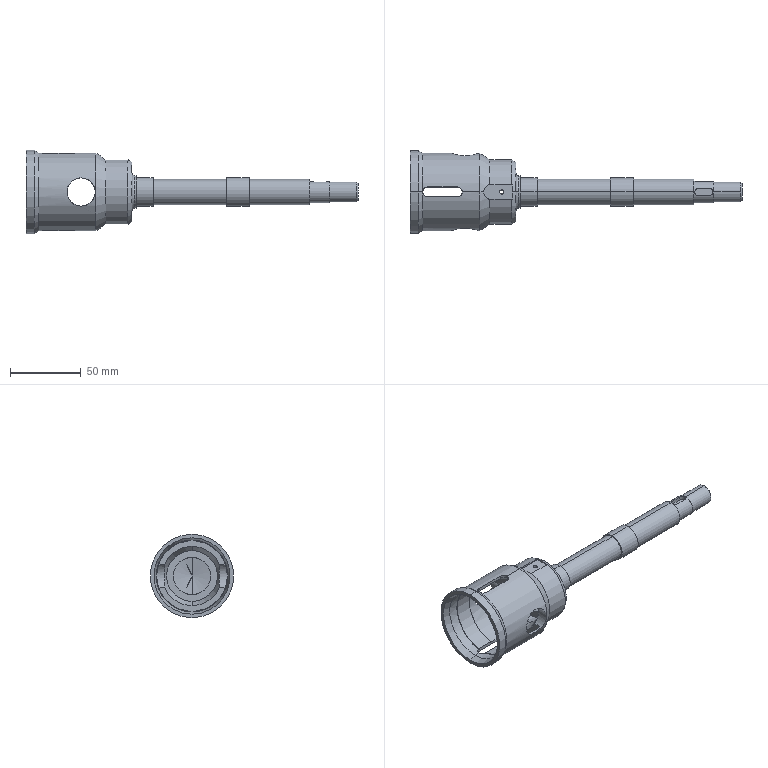Part | SolidWorks | features ICE 4, MirrorPattern 1, Revolution 1 | 1 solid | 97 faces | box 235 x 59 x 59 mm | volume 87330 mm3 | cylinder 50 | plane 31 | cone 14 | torus 2 | commonest cylinder face diameters 20 x8 7 x6 3 x4 18 x4 51 x4 5 x3